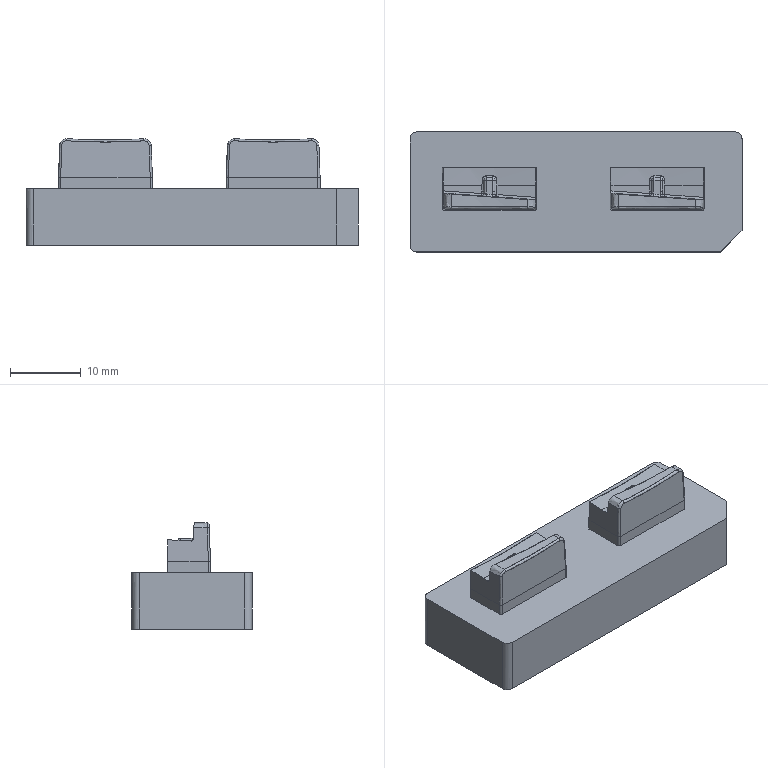NC program | PowerMill | posted with a generic post | part box 47 x 17 x 15.061 mm
Lines 1 to 1053 of 128250:
%
O0001
N104 ( POWERMILL CB  : 2026004.0)
N105 ( POST VER      : 2026.0.0.5161)
N106 ( OPTION FILE   : FANUC)
N107 ( OUTPUT WORKPLANE : WORLD)
N108 (  )
N109 ( TOOL LIST )
N110 (---------------------------------------)
N111 ( NO. | ID        | DIA.| TIP RAD|LENGTH)
N112 (---------------------------------------)
N113 (    1|D10C_1_1   |10.0 |  0.0   |70.52 )
N114 (    2|D4C_2_1    | 4.0 |  0.0   |62.12 )
N115 (   27|D1C_1_1    | 1.0 |  0.0   |58.04 )
N116 (    3|D10_1_1    |10.0 |  0.0   |70.24 )
N117 (    4|R1_2_1     | 2.0 |  1.0   |61.68 )
N118 (    6|R0.5_2_1   | 1.0 |  0.5   |58.12 )
N119 (   25|R0.3_1_1   | 0.6 |  0.3   |58.08 )
N120 (   13|TEXT_D4_1_1| 4.0 |  0.3   |62.32 )
N121 (---------------------------------------)
N122 (  )
N123 ( NUMBER OF TOOLPATHS: 13.0 )
N124 ( ESTIMATED PROGRAM DURATION: 0 HOURS 17 MIN 12 SEC)
N125 (  )
N126 G00 G21 G80 G40 G17
N127 G90
N128 G54
N129 G53 Z0.0
N130 (---------------)
N131 ( START TOOLPATH : 粗公开粗01-扫面平行-D10C )
N132 (---------------)
N133 ( TOOL NO.    :1 )
N134 ( TOOL TYPE   : ENDMILL)
N135 ( TOOL ID     : D10C_1_1)
N136 ( TOOL DIA    : 10.0 LENGTH 70.52)
N137 T1
N138 M6
N139 S8000 M03
N140 G00 G90 X0.0 Y0.0
N141 G43 Z10.2 H1
N142
N143 G05 P10000 R4
N144 X31.15 Y11.15
N145 Z1.001
N146 G01 Z-0.199 F6000.0
N147 X26.15 F10000.0
N148 X-26.15
N149 Y5.575
N150 X26.15
N151 Y0.0
N152 X-26.15
N153 Y-5.575
N154 X26.15
N155 Y-11.15
N156 X-26.15
N157 X-31.15
N158 G00 Z10.2
N159 G05 P0
N160 (---------------)
N161 ( END TOOLPATH : 粗公开粗01-扫面平行-D10C )
N162 (---------------)
N163 ( START TOOLPATH : 粗公开粗01-外形偏置-D10C )
N164 (---------------)
N165 G00 X-0.2 Y0.0 Z9.8009
N166 G05 P10000 R4
N167 X31.425 Y3.9948
N168 Z0.5886
N169 G01 Z-0.6113 F6000.0
N170 X30.8975 F10000.0
N171 G03 X26.15 Y-0.7527 I0.0 J-4.7475
N172 G01 Y-10.15
N173 G02 X25.15 Y-11.15 I-1.0 J0.0
N174 G01 X-25.55
N175 G02 X-26.55 Y-10.15 I0.0 J1.0
N176 G01 Y10.15
N177 G02 X-25.55 Y11.15 I1.0 J0.0
N178 G01 X25.15
N179 G02 X26.15 Y10.15 I0.0 J-1.0
N180 G01 Y-0.7527
N181 X22.8651 Y-0.7734
N182 X22.8749 Y-2.3203
N183 X22.7893 Y-3.0937
N184 X22.5905 Y-3.8671
N185 X22.2629 Y-4.6406
N186 X21.7652 Y-5.414
N187 X21.4559 Y-5.7792
N188 X21.0477 Y-6.1874
N189 X20.6825 Y-6.4854
N190 X19.908 Y-6.9608
N191 X19.1357 Y-7.2853
N192 X18.3622 Y-7.486
N193 X17.5888 Y-7.5756
N194 X11.4014 Y-7.5608
N195 X11.3997
N196 X5.9874 Y-7.5845
N197 X5.214 Y-7.5657
N198 X4.4406 Y-7.4607
N199 X3.6671 Y-7.2373
N200 X3.0301 Y-6.9608
N201 X2.1203 Y-6.3807
N202 X1.8907 Y-6.1874
N203 X1.3469 Y-5.6211
N204 X1.1772 Y-5.414
N205 X0.6795 Y-4.6406
N206 X0.3525 Y-3.8671
N207 X0.149 Y-3.0937
N208 X0.0636 Y-2.3203
N209 X0.0639 Y-2.1213
N210 X-0.8706 Y-2.1269
N211 X-0.8694 Y-2.3203
N212 X-0.9549 Y-3.0937
N213 X-1.1535 Y-3.8671
N214 X-1.4811 Y-4.6406
N215 X-1.7469 Y-5.0904
N216 X-1.9787 Y-5.414
N217 X-2.5203 Y-6.0221
N218 X-2.6962 Y-6.1874
N219 X-3.2937 Y-6.6483
N220 X-3.8363 Y-6.9608
N221 X-4.0671 Y-7.0697
N222 X-4.8406 Y-7.3592
N223 X-5.614 Y-7.5222
N224 X-6.3874 Y-7.5829
N225 X-12.5748 Y-7.5618
N226 X-12.5767
N227 X-17.9888 Y-7.5841
N228 X-18.7622 Y-7.5428
N229 X-19.5357 Y-7.4071
N230 X-20.3091 Y-7.1441
N231 X-20.7138 Y-6.9608
N232 X-21.0825 Y-6.7575
N233 X-21.8559 Y-6.1847
N234 X-22.5668 Y-5.414
N235 X-23.0644 Y-4.6406
N236 X-23.392 Y-3.8671
N237 X-23.5947 Y-3.0937
N238 X-23.6803 Y-2.3203
N239 X-23.6774 Y0.0
N240 X-23.5784 Y0.7734
N241 X-23.4028 Y1.41
N242 X-22.9881 Y2.3203
N243 X-22.6294 Y2.8555
N244 X-22.4379 Y3.0937
N245 X-21.8559 Y3.6697
N246 X-21.6074 Y3.8671
N247 X-21.0825 Y4.2097
N248 X-20.3091 Y4.5689
N249 X-19.5357 Y4.7862
N250 X-18.7622 Y4.879
N251 X-17.9888 Y4.8589
N252 X-5.614 Y3.9937
N253 X-4.8091 Y3.8671
N254 X-4.0671 Y3.6262
N255 X-3.2937 Y3.2321
N256 X-3.0826 Y3.0937
N257 X-2.5203 Y2.6427
N258 X-2.2009 Y2.3203
N259 X-1.7469 Y1.7402
N260 X-1.6216 Y1.5469
N261 X-1.234 Y0.7734
N262 X-0.9934 Y0.0
N263 X-0.8788 Y-0.7734
N264 X-0.8706 Y-2.1269
N265 X0.0639 Y-2.1213
N266 X0.0666 Y0.0
N267 X0.1669 Y0.7734
N268 X0.3891 Y1.5469
N269 X0.5734 Y1.975
N270 X0.7559 Y2.3203
N271 X1.3062 Y3.0937
N272 X2.1203 Y3.8547
N273 X2.8937 Y4.334
N274 X3.6432 Y4.6406
N275 X4.4406 Y4.8268
N276 X5.214 Y4.8845
N277 X5.9874 Y4.8431
N278 X17.5888 Y4.0317
N279 X18.3622 Y3.9708
N280 X19.1357 Y3.813
N281 X19.9091 Y3.5257
N282 X20.6825 Y3.0789
N283 X21.4559 Y2.4139
N284 X22.1221 Y1.5469
N285 X22.5098 Y0.7734
N286 X22.7505 Y0.0
N287 X22.8651 Y-0.7734
N288 X26.15 Y-0.7527
N289 G00 Z3.2763
N290 G01 X31.425 Y3.9948
N291 G00 Z0.2263
N292 G01 Z-0.9737 F6000.0
N293 X30.8975 F10000.0
N294 G03 X26.15 Y-0.7527 I0.0 J-4.7475
N295 G01 Y-0.7595
N296 X23.0634 Y-0.7734
N297 X23.0703 Y-2.3203
N298 X23.0028 Y-2.9944
N299 X22.793 Y-3.8671
N300 X22.4664 Y-4.6406
N301 X22.2294 Y-5.0499
N302 X21.9787 Y-5.414
N303 X21.4559 Y-6.0196
N304 X21.2786 Y-6.1874
N305 X20.6825 Y-6.6503
N306 X20.1695 Y-6.9608
N307 X19.9091 Y-7.0919
N308 X19.1357 Y-7.3812
N309 X18.3622 Y-7.542
N310 X17.5888 Y-7.599
N311 X5.214 Y-7.5973
N312 X4.4406 Y-7.5252
N313 X3.6671 Y-7.3398
N314 X2.8937 Y-7.0244
N315 X2.1203 Y-6.5627
N316 X1.6584 Y-6.1874
N317 X1.3469 Y-5.8804
N318 X0.9527 Y-5.414
N319 X0.5734 Y-4.8343
N320 X0.1477 Y-3.8671
N321 X-0.0447 Y-3.0937
N322 X-0.1307 Y-2.3203
N323 Y-2.1245
N324 X-0.6743 Y-2.1269
N325 X-0.6734 Y-2.3203
N326 X-0.7573 Y-3.0937
N327 X-0.9512 Y-3.8671
N328 X-1.2766 Y-4.6406
N329 X-1.7652 Y-5.414
N330 X-2.4653 Y-6.1874
N331 X-3.2937 Y-6.7976
N332 X-3.5744 Y-6.9608
N333 X-4.0671 Y-7.1938
N334 X-4.8406 Y-7.4403
N335 X-5.614 Y-7.5717
N336 X-6.3874 Y-7.5991
N337 X-17.9888
N338 X-18.7622 Y-7.5855
N339 X-19.5357 Y-7.4819
N340 X-20.3091 Y-7.2607
N341 X-20.9814 Y-6.9608
N342 X-21.8559 Y-6.3815
N343 X-22.0856 Y-6.1874
N344 X-22.6294 Y-5.6185
N345 X-22.7912 Y-5.414
N346 X-23.2747 Y-4.6406
N347 X-23.4028 Y-4.3721
N348 X-23.5956 Y-3.8671
N349 X-23.7947 Y-3.0937
N350 X-23.873 Y-2.3203
N351 X-23.8728 Y0.0
N352 X-23.7789 Y0.7734
N353 X-23.5578 Y1.5469
N354 X-23.4028 Y1.9231
N355 X-23.1996 Y2.3203
N356 X-22.6526 Y3.0937
N357 X-21.8384 Y3.8671
N358 X-21.0825 Y4.3381
N359 X-20.3767 Y4.6406
N360 X-19.5357 Y4.8446
N361 X-18.7622 Y4.9102
N362 X-17.9888 Y4.8716
N363 X-5.614 Y4.0075
N364 X-4.8406 Y3.9138
N365 X-4.0671 Y3.7005
N366 X-3.2937 Y3.3468
N367 X-2.8887 Y3.0937
N368 X-2.5203 Y2.8139
N369 X-2.0047 Y2.3203
N370 X-1.7469 Y2.0118
N371 X-1.4257 Y1.5469
N372 X-1.0365 Y0.7734
N373 X-0.7959 Y0.0
N374 X-0.6803 Y-0.7734
N375 X-0.6743 Y-2.1269
N376 X-0.1307 Y-2.1245
N377 X-0.1305 Y0.0
N378 X-0.0304 Y0.7734
N379 X0.1829 Y1.5469
N380 X0.5465 Y2.3203
N381 X1.0899 Y3.0937
N382 X1.3469 Y3.3723
N383 X1.9095 Y3.8671
N384 X2.1203 Y4.0175
N385 X2.8937 Y4.4526
N386 X3.3677 Y4.6406
N387 X3.6671 Y4.7291
N388 X4.4406 Y4.8759
N389 X5.214 Y4.9061
N390 X5.9874 Y4.8558
N391 X18.3622 Y3.989
N392 X19.1231 Y3.8671
N393 X19.9091 Y3.6108
N394 X20.6825 Y3.2077
N395 X20.8549 Y3.0937
N396 X21.4559 Y2.6073
N397 X21.7386 Y2.3203
N398 X22.2294 Y1.6887
N399 X22.7063 Y0.7734
N400 X22.9472 Y0.0
N401 X23.0634 Y-0.7734
N402 X26.15 Y-0.7595
N403 Y-10.15
N404 G02 X25.15 Y-11.15 I-1.0 J0.0
N405 G01 X-25.55
N406 G02 X-26.55 Y-10.15 I0.0 J1.0
N407 G01 Y10.15
N408 G02 X-25.55 Y11.15 I1.0 J0.0
N409 G01 X25.15
N410 G02 X26.15 Y10.15 I0.0 J-1.0
N411 G01 Y-0.7527
N412 G00 Z2.9139
N413 G01 X31.425 Y3.9948
N414 G00 Z-0.1361
N415 G01 Z-1.3361 F6000.0
N416 X30.8975 F10000.0
N417 G03 X26.15 Y-0.7527 I0.0 J-4.7475
N418 G01 Y-0.7529
N419 X23.1093 Y-0.7734
N420 X23.1198 Y-2.3203
N421 X23.0366 Y-3.0937
N422 X22.846 Y-3.8671
N423 X22.525 Y-4.6406
N424 X22.2294 Y-5.1497
N425 X22.0424 Y-5.414
N426 X21.4559 Y-6.0769
N427 X20.6825 Y-6.7039
N428 X20.2549 Y-6.9608
N429 X19.9091 Y-7.1302
N430 X19.1357 Y-7.4071
N431 X18.3622 Y-7.565
N432 X17.5888 Y-7.6116
N433 X5.214 Y-7.6106
N434 X4.4406 Y-7.5389
N435 X3.6671 Y-7.3585
N436 X2.8937 Y-7.0495
N437 X2.1203 Y-6.5828
N438 X1.6317 Y-6.1874
N439 X1.3469 Y-5.9085
N440 X0.9336 Y-5.414
N441 X0.5734 Y-4.8685
N442 X0.4501 Y-4.6406
N443 X0.1294 Y-3.8671
N444 X-0.062 Y-3.0937
N445 X-0.1442 Y-2.3203
N446 Y-1.7375
N447 X-0.628 Y-1.7402
N448 X-0.6247 Y-2.3203
N449 X-0.7069 Y-3.0937
N450 X-0.9016 Y-3.8671
N451 X-1.2195 Y-4.6406
N452 X-1.7016 Y-5.414
N453 X-2.4062 Y-6.1874
N454 X-3.2937 Y-6.8506
N455 X-3.4889 Y-6.9608
N456 X-4.0671 Y-7.2267
N457 X-4.8406 Y-7.4628
N458 X-5.614 Y-7.5903
N459 X-6.3874 Y-7.6117
N460 X-17.9888
N461 X-18.7622 Y-7.6016
N462 X-19.5357 Y-7.4946
N463 X-20.3091 Y-7.2808
N464 X-21.0232 Y-6.9608
N465 X-21.8559 Y-6.4048
N466 X-22.1123 Y-6.1874
N467 X-22.6294 Y-5.6451
N468 X-22.8103 Y-5.414
N469 X-23.2939 Y-4.6406
N470 X-23.6146 Y-3.8671
N471 X-23.806 Y-3.0937
N472 X-23.888 Y-2.3203
N473 X-23.8882 Y0.0
N474 X-23.7954 Y0.7734
N475 X-23.5786 Y1.5469
N476 X-23.4028 Y1.9675
N477 X-23.2201 Y2.3203
N478 X-22.681 Y3.0937
N479 X-21.8696 Y3.8671
N480 X-21.0825 Y4.3627
N481 X-20.4302 Y4.6406
N482 X-19.5357 Y4.8634
N483 X-18.7622 Y4.9247
N484 X-17.9888 Y4.8844
N485 X-5.614 Y4.02
N486 X-4.8406 Y3.9322
N487 X-4.5352 Y3.8671
N488 X-4.0671 Y3.7279
N489 X-3.2937 Y3.3831
N490 X-2.8271 Y3.0937
N491 X-2.5203 Y2.862
N492 X-1.949 Y2.3203
N493 X-1.7469 Y2.0824
N494 X-1.372 Y1.5469
N495 X-0.9734 Y0.7419
N496 X-0.7477 Y0.0
N497 X-0.6334 Y-0.7734
N498 X-0.628 Y-1.7402
N499 X-0.1442 Y-1.7375
N500 X-0.1443 Y0.0
N501 X-0.0515 Y0.7734
N502 X0.1653 Y1.5469
N503 X0.5239 Y2.3203
N504 X1.0628 Y3.0937
N505 X1.3469 Y3.4039
N506 X1.8744 Y3.8671
N507 X2.1203 Y4.0439
N508 X2.8937 Y4.4741
N509 X3.3137 Y4.6406
N510 X3.6671 Y4.7491
N511 X4.4406 Y4.8942
N512 X5.214 Y4.9205
N513 X18.3622 Y4.002
N514 X19.1357 Y3.8848
N515 X19.9091 Y3.6395
N516 X20.6825 Y3.247
N517 X20.9169 Y3.0937
N518 X21.4559 Y2.6615
N519 X21.7949 Y2.3203
N520 X22.2294 Y1.7678
N521 X22.3714 Y1.5469
N522 X22.7581 Y0.7734
N523 X22.9976 Y0.0
N524 X23.1093 Y-0.7734
N525 X26.15 Y-0.7529
N526 Y-10.15
N527 G02 X25.15 Y-11.15 I-1.0 J0.0
N528 G01 X-25.55
N529 G02 X-26.55 Y-10.15 I0.0 J1.0
N530 G01 Y10.15
N531 G02 X-25.55 Y11.15 I1.0 J0.0
N532 G01 X25.15
N533 G02 X26.15 Y10.15 I0.0 J-1.0
N534 G01 Y-0.7527
N535 G00 Z2.5516
N536 G01 X31.425 Y3.9948
N537 G00 Z-0.4984
N538 G01 Z-1.6984 F6000.0
N539 X30.8975 F10000.0
N540 G03 X26.15 Y-0.7527 I0.0 J-4.7475
N541 G01 Y-0.758
N542 X23.1247 Y-0.7734
N543 X23.1326 Y-2.3203
N544 X23.0522 Y-3.0937
N545 X22.859 Y-3.8671
N546 X22.5446 Y-4.6406
N547 X22.2294 Y-5.1814
N548 X22.0643 Y-5.414
N549 X21.4559 Y-6.0948
N550 X20.6825 Y-6.7247
N551 X20.2906 Y-6.9608
N552 X19.9091 Y-7.1483
N553 X19.1357 Y-7.4183
N554 X18.3622 Y-7.5795
N555 X17.5888 Y-7.6243
N556 X5.214 Y-7.6238
N557 X4.4406 Y-7.5535
N558 X3.6671 Y-7.3744
N559 X2.8937 Y-7.0682
N560 X2.685 Y-6.9608
N561 X2.1203 Y-6.6044
N562 X1.6069 Y-6.1874
N563 X1.3469 Y-5.9334
N564 X0.9117 Y-5.414
N565 X0.5734 Y-4.9026
N566 X0.4312 Y-4.6406
N567 X0.1137 Y-3.8671
N568 X-0.0768 Y-3.0937
N569 X-0.1571 Y-2.3203
N570 X-0.1572 Y-1.7379
N571 X-0.6142 Y-1.7402
N572 X-0.6113 Y-2.3203
N573 X-0.6917 Y-3.0937
N574 X-0.885 Y-3.8671
N575 X-1.1993 Y-4.6406
N576 X-1.6797 Y-5.414
N577 X-2.5203 Y-6.3109
N578 X-3.2937 Y-6.8706
N579 X-3.4534 Y-6.9608
N580 X-4.0671 Y-7.244
N581 X-4.8406 Y-7.4781
N582 X-5.614 Y-7.6044
N583 X-6.3874 Y-7.6244
N584 X-17.9888
N585 X-18.7622 Y-7.6149
N586 X-19.5357 Y-7.5095
N587 X-20.3091 Y-7.2974
N588 X-21.0825 Y-6.9482
N589 X-21.8559 Y-6.4262
N590 X-22.1371 Y-6.1874
N591 X-22.6294 Y-5.6723
N592 X-22.8322 Y-5.414
N593 X-23.3128 Y-4.6406
N594 X-23.6302 Y-3.8671
N595 X-23.8207 Y-3.0937
N596 X-23.9008 Y-2.3203
N597 X-23.9015 Y0.0
N598 X-23.8107 Y0.7734
N599 X-23.5962 Y1.5469
N600 X-23.4028 Y2.0076
N601 X-23.2404 Y2.3203
N602 X-22.705 Y3.0937
N603 X-21.9 Y3.8671
N604 X-21.0825 Y4.3827
N605 X-20.481 Y4.6406
N606 X-19.5357 Y4.8789
N607 X-18.7622 Y4.9383
N608 X-17.9888 Y4.8971
N609 X-5.614 Y4.0325
N610 X-4.8406 Y3.9465
N611 X-4.4751 Y3.8671
N612 X-4.0671 Y3.744
N613 X-3.2937 Y3.4017
N614 X-2.7976 Y3.0937
N615 X-2.5203 Y2.8846
N616 X-1.9258 Y2.3203
N617 X-1.7469 Y2.1098
N618 X-1.3518 Y1.5469
N619 X-0.9734 Y0.7856
N620 X-0.7309 Y0.0
N621 X-0.6192 Y-0.7734
N622 X-0.6142 Y-1.7402
N623 X-0.1572 Y-1.7379
N624 X-0.1575 Y0.0
N625 X-0.0668 Y0.7734
N626 X0.1477 Y1.5469
N627 X0.5035 Y2.3203
N628 X1.0387 Y3.0937
N629 X1.3469 Y3.4302
N630 X1.8441 Y3.8671
N631 X2.1203 Y4.0659
N632 X2.8937 Y4.4934
N633 X3.263 Y4.6406
N634 X3.6671 Y4.766
N635 X4.4406 Y4.9091
N636 X5.214 Y4.9337
N637 X18.3622 Y4.0151
N638 X19.1357 Y3.8995
N639 X19.9091 Y3.657
N640 X20.6825 Y3.2672
N641 X20.9463 Y3.0937
N642 X21.4559 Y2.6852
N643 X21.8181 Y2.3203
N644 X22.2294 Y1.798
N645 X22.3917 Y1.5469
N646 X22.7754 Y0.7734
N647 X23.0028 Y0.0436
N648 X23.1247 Y-0.7734
N649 X26.15 Y-0.758
N650 Y-10.15
N651 G02 X25.15 Y-11.15 I-1.0 J0.0
N652 G01 X-25.55
N653 G02 X-26.55 Y-10.15 I0.0 J1.0
N654 G01 Y10.15
N655 G02 X-25.55 Y11.15 I1.0 J0.0
N656 G01 X25.15
N657 G02 X26.15 Y10.15 I0.0 J-1.0
N658 G01 Y-0.7527
N659 G00 Z2.1892
N660 G01 X31.425 Y3.9948
N661 G00 Z-0.8608
N662 G01 Z-2.0608 F6000.0
N663 X30.8975 F10000.0
N664 G03 X26.15 Y-0.7527 I0.0 J-4.7475
N665 G01 Y-0.7597
N666 X23.1384 Y-0.7734
N667 X23.1455 Y-2.3203
N668 X23.0669 Y-3.0937
N669 X22.8755 Y-3.8671
N670 X22.5634 Y-4.6406
N671 X22.2294 Y-5.2124
N672 X22.0863 Y-5.414
N673 X21.4559 Y-6.1199
N674 X20.6825 Y-6.7455
N675 X20.326 Y-6.9608
N676 X19.9091 Y-7.1663
N677 X19.1357 Y-7.4343
N678 X18.3622 Y-7.5937
N679 X17.5888 Y-7.637
N680 X5.214 Y-7.6365
N681 X4.4406 Y-7.5681
N682 X3.6671 Y-7.3902
N683 X2.8937 Y-7.0869
N684 X2.6496 Y-6.9608
N685 X2.1203 Y-6.6259
N686 X1.5821 Y-6.1874
N687 X1.3469 Y-5.9582
N688 X0.8899 Y-5.414
N689 X0.5734 Y-4.9368
N690 X0.4124 Y-4.6406
N691 X0.098 Y-3.8671
N692 X-0.0915 Y-3.0937
N693 X-0.1701 Y-2.3203
N694 X-0.1702 Y-1.9317
N695 X-0.6001 Y-1.9336
N696 X-0.5984 Y-2.3203
N697 X-0.677 Y-3.0937
N698 X-0.8686 Y-3.8671
N699 X-0.9734 Y-4.1692
N700 X-1.1805 Y-4.6406
N701 X-1.7469 Y-5.5304
N702 X-2.5203 Y-6.3343
N703 X-3.418 Y-6.9608
N704 X-4.0671 Y-7.2614
N705 X-4.8406 Y-7.4937
N706 X-5.614 Y-7.6184
N707 X-6.3874 Y-7.637
N708 X-17.9888
N709 X-18.7622 Y-7.6281
N710 X-19.5357 Y-7.5246
N711 X-20.3091 Y-7.3141
N712 X-21.0825 Y-6.9677
N713 X-21.8559 Y-6.4488
N714 X-22.1619 Y-6.1874
N715 X-22.6294 Y-5.6996
N716 X-22.854 Y-5.414
N717 X-23.3318 Y-4.6406
N718 X-23.6459 Y-3.8671
N719 X-23.8354 Y-3.0937
N720 X-23.9137 Y-2.3203
N721 X-23.9147 Y0.0
N722 X-23.826 Y0.7734
N723 X-23.6138 Y1.5469
N724 X-23.4028 Y2.0476
N725 X-23.2607 Y2.3203
N726 X-22.7291 Y3.0937
N727 X-21.9304 Y3.8671
N728 X-21.0825 Y4.4027
N729 X-20.3091 Y4.7161
N730 X-19.5357 Y4.8944
N731 X-18.7622 Y4.9519
N732 X-17.9888 Y4.9099
N733 X-5.614 Y4.0451
N734 X-4.8406 Y3.9609
N735 X-4.4184 Y3.8671
N736 X-4.0671 Y3.7602
N737 X-3.2937 Y3.4204
N738 X-2.7682 Y3.0937
N739 X-2.5203 Y2.9066
N740 X-1.9026 Y2.3203
N741 X-1.7469 Y2.1373
N742 X-1.3317 Y1.5469
N743 X-0.9734 Y0.8286
N744 X-0.7155 Y0.0
N745 X-0.6053 Y-0.7734
N746 X-0.6001 Y-1.9336
N747 X-0.1702 Y-1.9317
N748 X-0.1708 Y0.0
N749 X-0.0821 Y0.7734
N750 X0.1301 Y1.5469
N751 X0.4832 Y2.3203
N752 X1.0145 Y3.0937
N753 X1.3469 Y3.4564
N754 X1.8139 Y3.8671
N755 X2.1203 Y4.088
N756 X2.8937 Y4.5127
N757 X3.2127 Y4.6406
N758 X3.6671 Y4.7829
N759 X4.4406 Y4.924
N760 X5.214 Y4.947
N761 X18.3622 Y4.0281
N762 X19.1357 Y3.9142
N763 X19.9091 Y3.6739
N764 X20.6825 Y3.2868
N765 X20.9757 Y3.0937
N766 X21.4559 Y2.7085
N767 X21.8413 Y2.3203
N768 X22.2294 Y1.8281
N769 X22.4115 Y1.5469
N770 X22.7927 Y0.7734
N771 X23.0028 Y0.1093
N772 X23.1384 Y-0.7734
N773 X26.15 Y-0.7597
N774 Y-10.15
N775 G02 X25.15 Y-11.15 I-1.0 J0.0
N776 G01 X-25.55
N777 G02 X-26.55 Y-10.15 I0.0 J1.0
N778 G01 Y10.15
N779 G02 X-25.55 Y11.15 I1.0 J0.0
N780 G01 X25.15
N781 G02 X26.15 Y10.15 I0.0 J-1.0
N782 G01 Y-0.7527
N783 G00 Z1.8268
N784 G01 X31.425 Y3.9948
N785 G00 Z-1.2232
N786 G01 Z-2.4232 F6000.0
N787 X30.8975 F10000.0
N788 G03 X26.15 Y-0.7527 I0.0 J-4.7475
N789 G01 Y-0.7614
N790 X23.1521 Y-0.7734
N791 X23.1583 Y-2.3203
N792 X23.0817 Y-3.0937
N793 X22.892 Y-3.8671
N794 X22.5822 Y-4.6406
N795 X22.1082 Y-5.414
N796 X21.4559 Y-6.1449
N797 X20.6825 Y-6.7663
N798 X20.3614 Y-6.9608
N799 X19.9091 Y-7.1844
N800 X19.1357 Y-7.4502
N801 X18.3622 Y-7.6079
N802 X17.5888 Y-7.6496
N803 X5.214 Y-7.6492
N804 X4.4406 Y-7.5827
N805 X3.6671 Y-7.406
N806 X2.8937 Y-7.1055
N807 X2.6143 Y-6.9608
N808 X2.1203 Y-6.6475
N809 X1.5573 Y-6.1874
N810 X1.3469 Y-5.9831
N811 X0.868 Y-5.414
N812 X0.5734 Y-4.9709
N813 X0.3935 Y-4.6406
N814 X0.0823 Y-3.8671
N815 X-0.1063 Y-3.0937
N816 X-0.183 Y-2.3203
N817 X-0.1831 Y-2.1254
N818 X-0.5863 Y-2.1269
N819 X-0.5856 Y-2.3203
N820 X-0.6622 Y-3.0937
N821 X-0.8521 Y-3.8671
N822 X-0.9734 Y-4.215
N823 X-1.1617 Y-4.6406
N824 X-1.636 Y-5.414
N825 X-2.3329 Y-6.1874
N826 X-2.5203 Y-6.3577
N827 X-3.3825 Y-6.9608
N828 X-4.0671 Y-7.2787
N829 X-4.8406 Y-7.5092
N830 X-5.614 Y-7.6324
N831 X-6.3874 Y-7.6497
N832 X-17.9888
N833 X-18.7622 Y-7.6414
N834 X-19.5357 Y-7.5398
N835 X-20.3091 Y-7.3307
N836 X-21.0825 Y-6.9871
N837 X-21.8559 Y-6.4714
N838 X-22.1867 Y-6.1874
N839 X-22.6294 Y-5.7268
N840 X-22.8759 Y-5.414
N841 X-23.3507 Y-4.6406
N842 X-23.6616 Y-3.8671
N843 X-23.8502 Y-3.0937
N844 X-23.9265 Y-2.3203
N845 X-23.9281 Y0.0
N846 X-23.8422 Y0.7734
N847 X-23.6314 Y1.5469
N848 X-23.281 Y2.3203
N849 X-22.7538 Y3.0937
N850 X-22.6294 Y3.238
N851 X-21.9607 Y3.8671
N852 X-21.0825 Y4.4227
N853 X-20.3091 Y4.7343
N854 X-19.5357 Y4.9099
N855 X-18.7622 Y4.966
N856 X-13.9547 Y4.6406
N857 X-13.6283
N858 X-13.3483 Y4.6814
N859 X-12.5748 Y4.7179
N860 X-11.028 Y4.5966
N861 X-10.1252 Y4.3732
N862 X-10.082 Y4.3702
N863 X-5.614 Y4.0576
N864 X-4.8406 Y3.9752
N865 X-4.4251 Y3.8686
N866 X-4.4184 Y3.8671
N867 X-4.4136 Y3.8656
N868 X-4.0671 Y3.7767
N869 X-3.2937 Y3.4391
N870 X-2.7388 Y3.0937
N871 X-2.5203 Y2.9286
N872 X-1.8791 Y2.3203
N873 X-1.3115 Y1.5469
N874 X-0.9734 Y0.8716
N875 X-0.7001 Y0.0
N876 X-0.5914 Y-0.7734
N877 X-0.5863 Y-2.1269
N878 X-0.1831 Y-2.1254
N879 X-0.184 Y0.0
N880 X-0.0974 Y0.7734
N881 X0.1125 Y1.5469
N882 X0.462 Y2.3203
N883 X0.5734 Y2.51
N884 X0.9904 Y3.0937
N885 X1.3469 Y3.4826
N886 X1.7833 Y3.8671
N887 X2.1203 Y4.1106
N888 X2.8937 Y4.5321
N889 X3.6671 Y4.7999
N890 X4.4406 Y4.9389
N891 X5.214 Y4.9603
N892 X9.8545 Y4.6372
N893 X10.1429 Y4.6406
N894 X10.628 Y4.7047
N895 X11.4014 Y4.7061
N896 X12.2341 Y4.6406
N897 X12.9482 Y4.5555
N898 X13.7217 Y4.3656
N899 X13.7644 Y4.3626
N900 X18.3622 Y4.0412
N901 X19.1357 Y3.9294
N902 X19.9091 Y3.6907
N903 X20.6825 Y3.3063
N904 X21.005 Y3.0937
N905 X21.4559 Y2.7318
N906 X21.8646 Y2.3203
N907 X22.2294 Y1.8582
N908 X22.4317 Y1.5469
N909 X22.81 Y0.7734
N910 X23.0028 Y0.1722
N911 X23.1521 Y-0.7734
N912 X26.15 Y-0.7614
N913 Y-10.15
N914 G02 X25.15 Y-11.15 I-1.0 J0.0
N915 G01 X-25.55
N916 G02 X-26.55 Y-10.15 I0.0 J1.0
N917 G01 Y10.15
N918 G02 X-25.55 Y11.15 I1.0 J0.0
N919 G01 X25.15
N920 G02 X26.15 Y10.15 I0.0 J-1.0
N921 G01 Y-0.7527
N922 G00 Z1.4363
N923 G01 X31.425 Y3.9948
N924 G00 Z-1.6137
N925 G01 Z-2.8137 F6000.0
N926 X30.8975 F10000.0
N927 G03 X26.15 Y-0.7527 I0.0 J-4.7475
N928 G01 Y-10.15
N929 G02 X25.15 Y-11.15 I-1.0 J0.0
N930 G01 X-25.55
N931 G02 X-26.55 Y-10.15 I0.0 J1.0
N932 G01 Y10.15
N933 G02 X-25.55 Y11.15 I1.0 J0.0
N934 G01 X5.0156
N935 X5.1173 Y8.6022
N936 X5.214 Y8.606
N937 X7.5343
N938 X8.3077 Y8.5796
N939 X9.0811 Y8.4493
N940 X9.8545 Y8.1648
N941 X10.6842 Y7.7343
N942 X11.158 Y7.338
N943 G03 X11.8073 Y7.3447 I0.3207 J0.3836
N944 G01 X12.3169 Y7.7343
N945 X12.9482 Y8.08
N946 X13.7217 Y8.3962
N947 X14.1822 Y8.5077
N948 X14.4951 Y8.5541
N949 X15.2685 Y8.606
N950 X18.3622 Y8.5944
N951 X19.0333 Y8.5077
N952 X19.9091 Y8.2506
N953 X20.6825 Y7.8682
N954 X20.8986 Y7.7343
N955 X21.4559 Y7.3026
N956 X21.8036 Y6.9608
N957 X22.2294 Y6.4395
N958 X22.3959 Y6.1874
N959 X22.795 Y5.414
N960 X23.0028 Y4.8009
N961 X23.1635 Y3.8671
N962 X23.1812 Y3.0937
N963 X23.1721 Y-2.3203
N964 X23.0976 Y-3.0937
N965 X22.9097 Y-3.8671
N966 X22.6024 Y-4.6406
N967 X22.1319 Y-5.414
N968 X21.4559 Y-6.1719
N969 X20.6825 Y-6.7887
N970 X20.3996 Y-6.9608
N971 X19.9091 Y-7.2038
N972 X19.1357 Y-7.4674
N973 X18.3622 Y-7.6231
N974 X17.5888 Y-7.6633
N975 X5.214 Y-7.6629
N976 X4.4406 Y-7.5985
N977 X3.6671 Y-7.4231
N978 X2.8937 Y-7.1257
N979 X2.5762 Y-6.9608
N980 X2.1203 Y-6.6707
N981 X1.5305 Y-6.1874
N982 X1.3469 Y-6.009
N983 X0.8445 Y-5.414
N984 X0.5734 Y-5.0077
N985 X0.3732 Y-4.6406
N986 X0.0654 Y-3.8671
N987 X-0.1223 Y-3.0937
N988 X-0.197 Y-2.3203
N989 X-0.2055 Y3.0937
N990 Y3.0941
N991 X-0.5778 Y3.0937
N992 X-0.5718 Y-2.3203
N993 X-0.6463 Y-3.0937
N994 X-0.8344 Y-3.8671
N995 X-0.9734 Y-4.2643
N996 X-1.1414 Y-4.6406
N997 X-1.6125 Y-5.414
N998 X-1.7469 Y-5.5894
N999 X-2.3053 Y-6.1874
N1000 X-2.5203 Y-6.3829
N1001 X-3.3443 Y-6.9608
N1002 X-4.0671 Y-7.2974
N1003 X-4.8406 Y-7.5261
N1004 X-5.614 Y-7.6472
N1005 X-6.3874 Y-7.6633
N1006 X-17.9888
N1007 X-18.7622 Y-7.6557
N1008 X-19.5357 Y-7.5562
N1009 X-20.3091 Y-7.3486
N1010 X-21.0825 Y-7.0079
N1011 X-21.8559 Y-6.4958
N1012 X-22.2134 Y-6.1874
N1013 X-22.6294 Y-5.7562
N1014 X-22.8995 Y-5.414
N1015 X-23.3711 Y-4.6406
N1016 X-23.6785 Y-3.8671
N1017 X-23.866 Y-3.0937
N1018 X-23.9404 Y-2.3203
N1019 X-23.9315 Y3.8671
N1020 X-23.8119 Y4.6406
N1021 X-23.5632 Y5.414
N1022 X-23.4028 Y5.7659
N1023 X-23.1646 Y6.1874
N1024 X-22.6294 Y6.8986
N1025 X-21.8559 Y7.6012
N1026 X-21.6666 Y7.7343
N1027 X-21.0825 Y8.0717
N1028 X-20.3091 Y8.3765
N1029 X-19.8015 Y8.5077
N1030 X-19.5357 Y8.5511
N1031 X-18.7622 Y8.606
N1032 X-15.6685 Y8.6
N1033 X-14.8951 Y8.5068
N1034 X-14.1217 Y8.2756
N1035 X-13.0069 Y7.7343
N1036 X-12.6746 Y7.4519
N1037 X-12.6125 Y7.4069
N1038 X-12.5442 Y7.3719
N1039 G03 X-11.888 Y7.3917 I0.3167 J0.3869
N1040 G01 X-11.8014 Y7.4718
N1041 X-11.4318 Y7.7343
N1042 X-11.028 Y7.9715
N1043 X-10.2545 Y8.3194
N1044 X-9.6049 Y8.5077
N1045 X-8.7077 Y8.6037
N1046 X-5.614 Y8.605
N1047 X-4.8406 Y8.5301
N1048 X-4.0671 Y8.3337
N1049 X-3.2937 Y7.999
N1050 X-2.8459 Y7.7343
N1051 X-2.5203 Y7.4963
N1052 X-1.9388 Y6.9608
N1053 X-1.7469 Y6.7419
N1054 X-1.3481 Y6.1874
N1055 X-0.9734 Y5.4725
N1056 X-0.7003 Y4.6406
N1057 X-0.5787 Y3.8671
N1058 X-0.5778 Y3.0937
N1059 X-0.2055 Y3.0941
N1060 X-0.2 Y3.7035
N1061 X-0.0672 Y4.6406
N1062 X0.1811 Y5.414
N1063 X0.5734 Y6.1801
N1064 X1.1706 Y6.9608
N1065 X1.3469 Y7.1405
N1066 X2.079 Y7.7343
N1067 X2.8937 Y8.1791
N1068 X3.6671 Y8.441
N1069 X3.9434 Y8.5077
N1070 X4.4406 Y8.5751
N1071 X5.1173 Y8.6022
N1072 X5.0156 Y11.15
N1073 X25.15
N1074 G02 X26.15 Y10.15 I0.0 J-1.0
N1075 G01 Y-0.7527
N1076 G00 Z1.0457
N1077 G01 X31.425 Y3.9948
N1078 G00 Z-2.0043
N1079 G01 Z-3.2043 F6000.0
N1080 X30.8975 F10000.0
N1081 G03 X26.15 Y-0.7527 I0.0 J-4.7475
N1082 G01 Y-10.15
N1083 G02 X25.15 Y-11.15 I-1.0 J0.0
N1084 G01 X-25.55
N1085 G02 X-26.55 Y-10.15 I0.0 J1.0
N1086 G01 Y10.15
N1087 G02 X-25.55 Y11.15 I1.0 J0.0
N1088 G01 X4.363
N1089 X4.4406 Y8.5827
N1090 X5.214 Y8.606
N1091 X17.5888
N1092 X18.3622 Y8.5963
N1093 X19.0469 Y8.5077
N1094 X19.9091 Y8.2569
N1095 X20.6825 Y7.8794
N1096 X20.9122 Y7.7343
N1097 X21.4559 Y7.3147
N1098 X21.8188 Y6.9608
N1099 X22.2294 Y6.458
N1100 X22.4113 Y6.1874
N1101 X22.8086 Y5.414
N1102 X23.0573 Y4.6406
N1103 X23.1789 Y3.8671
N1104 X23.1948 Y3.0937
N1105 X23.186 Y-2.3203
N1106 X23.1135 Y-3.0937
N1107 X22.9275 Y-3.8671
N1108 X22.6227 Y-4.6406
N1109 X22.2294 Y-5.3099
N1110 X21.4676 Y-6.1874
N1111 X20.6825 Y-6.8111
N1112 X20.4377 Y-6.9608
N1113 X19.9091 Y-7.2232
N1114 X19.1357 Y-7.4846
N1115 X18.3622 Y-7.6384
N1116 X17.5888 Y-7.6769
N1117 X5.214 Y-7.6766
N1118 X4.4406 Y-7.6142
N1119 X3.6671 Y-7.4402
N1120 X2.8937 Y-7.1458
N1121 X2.5381 Y-6.9608
N1122 X2.1203 Y-6.694
N1123 X1.3469 Y-6.035
N1124 X0.8209 Y-5.414
N1125 X0.5734 Y-5.0445
N1126 X0.3529 Y-4.6406
N1127 X0.0479 Y-3.8671
N1128 X-0.1382 Y-3.0937
N1129 X-0.2108 Y-2.3203
N1130 X-0.2047 Y2.639
N1131 X-0.2054 Y3.0931
N1132 X-0.5491 Y3.0937
N1133 X-0.5579 Y-2.3203
N1134 X-0.6304 Y-3.0937
N1135 X-0.8167 Y-3.8671
N1136 X-0.9734 Y-4.311
N1137 X-1.1211 Y-4.6406
N1138 X-1.589 Y-5.414
N1139 X-1.7469 Y-5.6195
N1140 X-2.2776 Y-6.1874
N1141 X-2.5203 Y-6.4081
N1142 X-3.3061 Y-6.9608
N1143 X-4.0671 Y-7.316
N1144 X-4.8406 Y-7.5429
N1145 X-5.614 Y-7.6618
N1146 X-6.3874 Y-7.677
N1147 X-17.9888
N1148 X-18.7622 Y-7.67
N1149 X-19.5357 Y-7.5725
N1150 X-20.3091 Y-7.3665